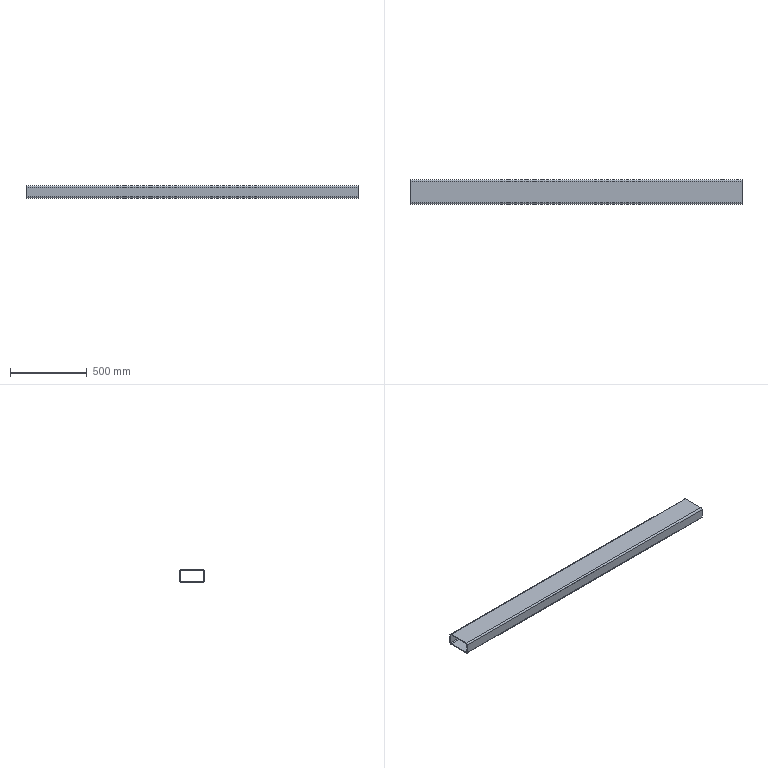Part | SolidWorks | features BaseBody 1 | 1 solid | 26 faces | box 2160 x 160 x 80 mm | volume 4825859 mm3 | cylinder 16 | plane 10 | commonest cylinder face diameters 14 x8 10 x4 20 x4
STEP:
#1=CARTESIAN_POINT('',(1050.,75.,-17.));
#2=VERTEX_POINT('',#1);
#3=CARTESIAN_POINT('',(1050.,75.,-3.));
#4=VERTEX_POINT('',#3);
#5=CARTESIAN_POINT('',(1050.,75.,-10.));
#6=DIRECTION('',(0.,-1.,0.));
#7=DIRECTION('',(0.,0.,-1.));
#8=AXIS2_PLACEMENT_3D('',#5,#6,#7);
#9=CIRCLE('',#8,7.);
#10=EDGE_CURVE('',#2,#4,#9,.T.);
#11=ORIENTED_EDGE('',*,*,#10,.T.);
#12=CARTESIAN_POINT('',(1050.,80.,-3.));
#13=VERTEX_POINT('',#12);
#14=CARTESIAN_POINT('',(1050.,100.,-3.));
#15=DIRECTION('',(0.,1.,0.));
#16=VECTOR('',#15,1000.);
#17=LINE('',#14,#16);
#18=EDGE_CURVE('',#4,#13,#17,.T.);
#19=ORIENTED_EDGE('',*,*,#18,.T.);
#20=CARTESIAN_POINT('',(1050.,80.,-17.));
#21=VERTEX_POINT('',#20);
#22=CARTESIAN_POINT('',(1050.,80.,-10.));
#23=DIRECTION('',(0.,-1.,0.));
#24=DIRECTION('',(0.,0.,-1.));
#25=AXIS2_PLACEMENT_3D('',#22,#23,#24);
#26=CIRCLE('',#25,7.);
#27=EDGE_CURVE('',#21,#13,#26,.T.);
#28=ORIENTED_EDGE('',*,*,#27,.F.);
#29=CARTESIAN_POINT('',(1050.,100.,-17.));
#30=DIRECTION('',(0.,1.,0.));
#31=VECTOR('',#30,1000.);
#32=LINE('',#29,#31);
#33=EDGE_CURVE('',#2,#21,#32,.T.);
#34=ORIENTED_EDGE('',*,*,#33,.F.);
#35=EDGE_LOOP('',(#11,#19,#28,#34));
#36=FACE_OUTER_BOUND('',#35,.T.);
#37=CARTESIAN_POINT('',(1050.,100.,-10.));
#38=DIRECTION('',(0.,1.,0.));
#39=DIRECTION('',(0.,0.,-1.));
#40=AXIS2_PLACEMENT_3D('',#37,#38,#39);
#41=CYLINDRICAL_SURFACE('',#40,7.);
#42=ADVANCED_FACE('',(#36),#41,.F.);
#43=CARTESIAN_POINT('',(950.,75.,-17.));
#44=VERTEX_POINT('',#43);
#45=CARTESIAN_POINT('',(950.,75.,-3.));
#46=VERTEX_POINT('',#45);
#47=CARTESIAN_POINT('',(950.,75.,-10.));
#48=DIRECTION('',(0.,-1.,0.));
#49=DIRECTION('',(0.,0.,-1.));
#50=AXIS2_PLACEMENT_3D('',#47,#48,#49);
#51=CIRCLE('',#50,7.);
#52=EDGE_CURVE('',#44,#46,#51,.T.);
#53=ORIENTED_EDGE('',*,*,#52,.T.);
#54=CARTESIAN_POINT('',(950.,80.,-3.));
#55=VERTEX_POINT('',#54);
#56=CARTESIAN_POINT('',(950.,100.,-3.));
#57=DIRECTION('',(0.,1.,0.));
#58=VECTOR('',#57,1000.);
#59=LINE('',#56,#58);
#60=EDGE_CURVE('',#46,#55,#59,.T.);
#61=ORIENTED_EDGE('',*,*,#60,.T.);
#62=CARTESIAN_POINT('',(950.,80.,-17.));
#63=VERTEX_POINT('',#62);
#64=CARTESIAN_POINT('',(950.,80.,-10.));
#65=DIRECTION('',(0.,-1.,0.));
#66=DIRECTION('',(0.,0.,-1.));
#67=AXIS2_PLACEMENT_3D('',#64,#65,#66);
#68=CIRCLE('',#67,7.);
#69=EDGE_CURVE('',#63,#55,#68,.T.);
#70=ORIENTED_EDGE('',*,*,#69,.F.);
#71=CARTESIAN_POINT('',(950.,100.,-17.));
#72=DIRECTION('',(0.,1.,0.));
#73=VECTOR('',#72,1000.);
#74=LINE('',#71,#73);
#75=EDGE_CURVE('',#44,#63,#74,.T.);
#76=ORIENTED_EDGE('',*,*,#75,.F.);
#77=EDGE_LOOP('',(#53,#61,#70,#76));
#78=FACE_OUTER_BOUND('',#77,.T.);
#79=CARTESIAN_POINT('',(950.,100.,-10.));
#80=DIRECTION('',(0.,1.,0.));
#81=DIRECTION('',(0.,0.,-1.));
#82=AXIS2_PLACEMENT_3D('',#79,#80,#81);
#83=CYLINDRICAL_SURFACE('',#82,7.);
#84=ADVANCED_FACE('',(#78),#83,.F.);
#85=CARTESIAN_POINT('',(-220.,75.,-17.));
#86=VERTEX_POINT('',#85);
#87=CARTESIAN_POINT('',(-220.,75.,-3.));
#88=VERTEX_POINT('',#87);
#89=CARTESIAN_POINT('',(-220.,75.,-10.));
#90=DIRECTION('',(0.,-1.,0.));
#91=DIRECTION('',(0.,0.,-1.));
#92=AXIS2_PLACEMENT_3D('',#89,#90,#91);
#93=CIRCLE('',#92,7.);
#94=EDGE_CURVE('',#86,#88,#93,.T.);
#95=ORIENTED_EDGE('',*,*,#94,.T.);
#96=CARTESIAN_POINT('',(-220.,80.,-3.));
#97=VERTEX_POINT('',#96);
#98=CARTESIAN_POINT('',(-220.,100.,-3.));
#99=DIRECTION('',(0.,1.,0.));
#100=VECTOR('',#99,1000.);
#101=LINE('',#98,#100);
#102=EDGE_CURVE('',#88,#97,#101,.T.);
#103=ORIENTED_EDGE('',*,*,#102,.T.);
#104=CARTESIAN_POINT('',(-220.,80.,-17.));
#105=VERTEX_POINT('',#104);
#106=CARTESIAN_POINT('',(-220.,80.,-10.));
#107=DIRECTION('',(0.,-1.,0.));
#108=DIRECTION('',(0.,0.,-1.));
#109=AXIS2_PLACEMENT_3D('',#106,#107,#108);
#110=CIRCLE('',#109,7.);
#111=EDGE_CURVE('',#105,#97,#110,.T.);
#112=ORIENTED_EDGE('',*,*,#111,.F.);
#113=CARTESIAN_POINT('',(-220.,100.,-17.));
#114=DIRECTION('',(0.,1.,0.));
#115=VECTOR('',#114,1000.);
#116=LINE('',#113,#115);
#117=EDGE_CURVE('',#86,#105,#116,.T.);
#118=ORIENTED_EDGE('',*,*,#117,.F.);
#119=EDGE_LOOP('',(#95,#103,#112,#118));
#120=FACE_OUTER_BOUND('',#119,.T.);
#121=CARTESIAN_POINT('',(-220.,100.,-10.));
#122=DIRECTION('',(0.,1.,0.));
#123=DIRECTION('',(0.,0.,-1.));
#124=AXIS2_PLACEMENT_3D('',#121,#122,#123);
#125=CYLINDRICAL_SURFACE('',#124,7.);
#126=ADVANCED_FACE('',(#120),#125,.F.);
#127=CARTESIAN_POINT('',(-320.,75.,-17.));
#128=VERTEX_POINT('',#127);
#129=CARTESIAN_POINT('',(-320.,75.,-3.));
#130=VERTEX_POINT('',#129);
#131=CARTESIAN_POINT('',(-320.,75.,-10.));
#132=DIRECTION('',(0.,-1.,0.));
#133=DIRECTION('',(0.,0.,-1.));
#134=AXIS2_PLACEMENT_3D('',#131,#132,#133);
#135=CIRCLE('',#134,7.);
#136=EDGE_CURVE('',#128,#130,#135,.T.);
#137=ORIENTED_EDGE('',*,*,#136,.T.);
#138=CARTESIAN_POINT('',(-320.,80.,-3.));
#139=VERTEX_POINT('',#138);
#140=CARTESIAN_POINT('',(-320.,100.,-3.));
#141=DIRECTION('',(0.,1.,0.));
#142=VECTOR('',#141,1000.);
#143=LINE('',#140,#142);
#144=EDGE_CURVE('',#130,#139,#143,.T.);
#145=ORIENTED_EDGE('',*,*,#144,.T.);
#146=CARTESIAN_POINT('',(-320.,80.,-17.));
#147=VERTEX_POINT('',#146);
#148=CARTESIAN_POINT('',(-320.,80.,-10.));
#149=DIRECTION('',(0.,-1.,0.));
#150=DIRECTION('',(0.,0.,-1.));
#151=AXIS2_PLACEMENT_3D('',#148,#149,#150);
#152=CIRCLE('',#151,7.);
#153=EDGE_CURVE('',#147,#139,#152,.T.);
#154=ORIENTED_EDGE('',*,*,#153,.F.);
#155=CARTESIAN_POINT('',(-320.,100.,-17.));
#156=DIRECTION('',(0.,1.,0.));
#157=VECTOR('',#156,1000.);
#158=LINE('',#155,#157);
#159=EDGE_CURVE('',#128,#147,#158,.T.);
#160=ORIENTED_EDGE('',*,*,#159,.F.);
#161=EDGE_LOOP('',(#137,#145,#154,#160));
#162=FACE_OUTER_BOUND('',#161,.T.);
#163=CARTESIAN_POINT('',(-320.,100.,-10.));
#164=DIRECTION('',(0.,1.,0.));
#165=DIRECTION('',(0.,0.,-1.));
#166=AXIS2_PLACEMENT_3D('',#163,#164,#165);
#167=CYLINDRICAL_SURFACE('',#166,7.);
#168=ADVANCED_FACE('',(#162),#167,.F.);
#169=CARTESIAN_POINT('',(-1080.,70.,-40.));
#170=VERTEX_POINT('',#169);
#171=CARTESIAN_POINT('',(-1080.,80.,-30.));
#172=VERTEX_POINT('',#171);
#173=CARTESIAN_POINT('',(-1080.,70.,-30.));
#174=DIRECTION('',(1.,0.,0.));
#175=DIRECTION('',(0.,0.,-1.));
#176=AXIS2_PLACEMENT_3D('',#173,#174,#175);
#177=CIRCLE('',#176,10.);
#178=EDGE_CURVE('',#170,#172,#177,.T.);
#179=ORIENTED_EDGE('',*,*,#178,.T.);
#180=CARTESIAN_POINT('',(1080.,80.,-30.));
#181=VERTEX_POINT('',#180);
#182=CARTESIAN_POINT('',(1080.,80.,-30.));
#183=DIRECTION('',(-1.,0.,0.));
#184=VECTOR('',#183,1000.);
#185=LINE('',#182,#184);
#186=EDGE_CURVE('',#181,#172,#185,.T.);
#187=ORIENTED_EDGE('',*,*,#186,.F.);
#188=CARTESIAN_POINT('',(1080.,70.,-40.));
#189=VERTEX_POINT('',#188);
#190=CARTESIAN_POINT('',(1080.,70.,-30.));
#191=DIRECTION('',(1.,0.,0.));
#192=DIRECTION('',(0.,0.,-1.));
#193=AXIS2_PLACEMENT_3D('',#190,#191,#192);
#194=CIRCLE('',#193,10.);
#195=EDGE_CURVE('',#189,#181,#194,.T.);
#196=ORIENTED_EDGE('',*,*,#195,.F.);
#197=CARTESIAN_POINT('',(1080.,70.,-40.));
#198=DIRECTION('',(-1.,0.,0.));
#199=VECTOR('',#198,1000.);
#200=LINE('',#197,#199);
#201=EDGE_CURVE('',#189,#170,#200,.T.);
#202=ORIENTED_EDGE('',*,*,#201,.T.);
#203=EDGE_LOOP('',(#179,#187,#196,#202));
#204=FACE_OUTER_BOUND('',#203,.T.);
#205=CARTESIAN_POINT('',(1080.,70.,-30.));
#206=DIRECTION('',(-1.,0.,0.));
#207=DIRECTION('',(0.,0.,1.));
#208=AXIS2_PLACEMENT_3D('',#205,#206,#207);
#209=CYLINDRICAL_SURFACE('',#208,10.);
#210=ADVANCED_FACE('',(#204),#209,.T.);
#211=ORIENTED_EDGE('',*,*,#27,.T.);
#212=CARTESIAN_POINT('',(1050.,80.,-10.));
#213=DIRECTION('',(0.,-1.,0.));
#214=DIRECTION('',(0.,0.,-1.));
#215=AXIS2_PLACEMENT_3D('',#212,#213,#214);
#216=CIRCLE('',#215,7.);
#217=EDGE_CURVE('',#13,#21,#216,.T.);
#218=ORIENTED_EDGE('',*,*,#217,.T.);
#219=EDGE_LOOP('',(#211,#218));
#220=FACE_BOUND('',#219,.T.);
#221=ORIENTED_EDGE('',*,*,#69,.T.);
#222=CARTESIAN_POINT('',(950.,80.,-10.));
#223=DIRECTION('',(0.,-1.,0.));
#224=DIRECTION('',(0.,0.,-1.));
#225=AXIS2_PLACEMENT_3D('',#222,#223,#224);
#226=CIRCLE('',#225,7.);
#227=EDGE_CURVE('',#55,#63,#226,.T.);
#228=ORIENTED_EDGE('',*,*,#227,.T.);
#229=EDGE_LOOP('',(#221,#228));
#230=FACE_BOUND('',#229,.T.);
#231=ORIENTED_EDGE('',*,*,#111,.T.);
#232=CARTESIAN_POINT('',(-220.,80.,-10.));
#233=DIRECTION('',(0.,-1.,0.));
#234=DIRECTION('',(0.,0.,-1.));
#235=AXIS2_PLACEMENT_3D('',#232,#233,#234);
#236=CIRCLE('',#235,7.);
#237=EDGE_CURVE('',#97,#105,#236,.T.);
#238=ORIENTED_EDGE('',*,*,#237,.T.);
#239=EDGE_LOOP('',(#231,#238));
#240=FACE_BOUND('',#239,.T.);
#241=ORIENTED_EDGE('',*,*,#153,.T.);
#242=CARTESIAN_POINT('',(-320.,80.,-10.));
#243=DIRECTION('',(0.,-1.,0.));
#244=DIRECTION('',(0.,0.,-1.));
#245=AXIS2_PLACEMENT_3D('',#242,#243,#244);
#246=CIRCLE('',#245,7.);
#247=EDGE_CURVE('',#139,#147,#246,.T.);
#248=ORIENTED_EDGE('',*,*,#247,.T.);
#249=EDGE_LOOP('',(#241,#248));
#250=FACE_BOUND('',#249,.T.);
#251=CARTESIAN_POINT('',(-1080.,80.,30.));
#252=VERTEX_POINT('',#251);
#253=CARTESIAN_POINT('',(-1080.,80.,-30.));
#254=DIRECTION('',(0.,0.,1.));
#255=VECTOR('',#254,1000.);
#256=LINE('',#253,#255);
#257=EDGE_CURVE('',#172,#252,#256,.T.);
#258=ORIENTED_EDGE('',*,*,#257,.T.);
#259=CARTESIAN_POINT('',(1080.,80.,30.));
#260=VERTEX_POINT('',#259);
#261=CARTESIAN_POINT('',(1080.,80.,30.));
#262=DIRECTION('',(-1.,0.,0.));
#263=VECTOR('',#262,1000.);
#264=LINE('',#261,#263);
#265=EDGE_CURVE('',#260,#252,#264,.T.);
#266=ORIENTED_EDGE('',*,*,#265,.F.);
#267=CARTESIAN_POINT('',(1080.,80.,-30.));
#268=DIRECTION('',(0.,0.,1.));
#269=VECTOR('',#268,1000.);
#270=LINE('',#267,#269);
#271=EDGE_CURVE('',#181,#260,#270,.T.);
#272=ORIENTED_EDGE('',*,*,#271,.F.);
#273=ORIENTED_EDGE('',*,*,#186,.T.);
#274=EDGE_LOOP('',(#258,#266,#272,#273));
#275=FACE_OUTER_BOUND('',#274,.T.);
#276=CARTESIAN_POINT('',(1080.,80.,-30.));
#277=DIRECTION('',(0.,-1.,0.));
#278=DIRECTION('',(0.,0.,-1.));
#279=AXIS2_PLACEMENT_3D('',#276,#277,#278);
#280=PLANE('',#279);
#281=ADVANCED_FACE('',(#220,#230,#240,#250,#275),#280,.F.);
#282=CARTESIAN_POINT('',(-1080.,70.,40.));
#283=VERTEX_POINT('',#282);
#284=CARTESIAN_POINT('',(-1080.,70.,30.));
#285=DIRECTION('',(1.,0.,0.));
#286=DIRECTION('',(0.,0.,-1.));
#287=AXIS2_PLACEMENT_3D('',#284,#285,#286);
#288=CIRCLE('',#287,10.);
#289=EDGE_CURVE('',#252,#283,#288,.T.);
#290=ORIENTED_EDGE('',*,*,#289,.T.);
#291=CARTESIAN_POINT('',(1080.,70.,40.));
#292=VERTEX_POINT('',#291);
#293=CARTESIAN_POINT('',(1080.,70.,40.));
#294=DIRECTION('',(-1.,0.,0.));
#295=VECTOR('',#294,1000.);
#296=LINE('',#293,#295);
#297=EDGE_CURVE('',#292,#283,#296,.T.);
#298=ORIENTED_EDGE('',*,*,#297,.F.);
#299=CARTESIAN_POINT('',(1080.,70.,30.));
#300=DIRECTION('',(1.,0.,0.));
#301=DIRECTION('',(0.,0.,-1.));
#302=AXIS2_PLACEMENT_3D('',#299,#300,#301);
#303=CIRCLE('',#302,10.);
#304=EDGE_CURVE('',#260,#292,#303,.T.);
#305=ORIENTED_EDGE('',*,*,#304,.F.);
#306=ORIENTED_EDGE('',*,*,#265,.T.);
#307=EDGE_LOOP('',(#290,#298,#305,#306));
#308=FACE_OUTER_BOUND('',#307,.T.);
#309=CARTESIAN_POINT('',(1080.,70.,30.));
#310=DIRECTION('',(-1.,0.,0.));
#311=DIRECTION('',(0.,0.,1.));
#312=AXIS2_PLACEMENT_3D('',#309,#310,#311);
#313=CYLINDRICAL_SURFACE('',#312,10.);
#314=ADVANCED_FACE('',(#308),#313,.T.);
#315=CARTESIAN_POINT('',(-1080.,-70.,40.));
#316=VERTEX_POINT('',#315);
#317=CARTESIAN_POINT('',(-1080.,-70.,40.));
#318=DIRECTION('',(0.,-1.,0.));
#319=VECTOR('',#318,1000.);
#320=LINE('',#317,#319);
#321=EDGE_CURVE('',#283,#316,#320,.T.);
#322=ORIENTED_EDGE('',*,*,#321,.T.);
#323=CARTESIAN_POINT('',(1080.,-70.,40.));
#324=VERTEX_POINT('',#323);
#325=CARTESIAN_POINT('',(1080.,-70.,40.));
#326=DIRECTION('',(-1.,0.,0.));
#327=VECTOR('',#326,1000.);
#328=LINE('',#325,#327);
#329=EDGE_CURVE('',#324,#316,#328,.T.);
#330=ORIENTED_EDGE('',*,*,#329,.F.);
#331=CARTESIAN_POINT('',(1080.,-70.,40.));
#332=DIRECTION('',(0.,-1.,0.));
#333=VECTOR('',#332,1000.);
#334=LINE('',#331,#333);
#335=EDGE_CURVE('',#292,#324,#334,.T.);
#336=ORIENTED_EDGE('',*,*,#335,.F.);
#337=ORIENTED_EDGE('',*,*,#297,.T.);
#338=EDGE_LOOP('',(#322,#330,#336,#337));
#339=FACE_OUTER_BOUND('',#338,.T.);
#340=CARTESIAN_POINT('',(1080.,-70.,40.));
#341=DIRECTION('',(0.,0.,-1.));
#342=DIRECTION('',(0.,1.,0.));
#343=AXIS2_PLACEMENT_3D('',#340,#341,#342);
#344=PLANE('',#343);
#345=ADVANCED_FACE('',(#339),#344,.F.);
#346=CARTESIAN_POINT('',(-1080.,-80.,30.));
#347=VERTEX_POINT('',#346);
#348=CARTESIAN_POINT('',(-1080.,-70.,30.));
#349=DIRECTION('',(1.,0.,0.));
#350=DIRECTION('',(0.,0.,-1.));
#351=AXIS2_PLACEMENT_3D('',#348,#349,#350);
#352=CIRCLE('',#351,10.);
#353=EDGE_CURVE('',#316,#347,#352,.T.);
#354=ORIENTED_EDGE('',*,*,#353,.T.);
#355=CARTESIAN_POINT('',(1080.,-80.,30.));
#356=VERTEX_POINT('',#355);
#357=CARTESIAN_POINT('',(1080.,-80.,30.));
#358=DIRECTION('',(-1.,0.,0.));
#359=VECTOR('',#358,1000.);
#360=LINE('',#357,#359);
#361=EDGE_CURVE('',#356,#347,#360,.T.);
#362=ORIENTED_EDGE('',*,*,#361,.F.);
#363=CARTESIAN_POINT('',(1080.,-70.,30.));
#364=DIRECTION('',(1.,0.,0.));
#365=DIRECTION('',(0.,0.,-1.));
#366=AXIS2_PLACEMENT_3D('',#363,#364,#365);
#367=CIRCLE('',#366,10.);
#368=EDGE_CURVE('',#324,#356,#367,.T.);
#369=ORIENTED_EDGE('',*,*,#368,.F.);
#370=ORIENTED_EDGE('',*,*,#329,.T.);
#371=EDGE_LOOP('',(#354,#362,#369,#370));
#372=FACE_OUTER_BOUND('',#371,.T.);
#373=CARTESIAN_POINT('',(1080.,-70.,30.));
#374=DIRECTION('',(-1.,0.,0.));
#375=DIRECTION('',(0.,0.,1.));
#376=AXIS2_PLACEMENT_3D('',#373,#374,#375);
#377=CYLINDRICAL_SURFACE('',#376,10.);
#378=ADVANCED_FACE('',(#372),#377,.T.);
#379=CARTESIAN_POINT('',(-1080.,-80.,-30.));
#380=VERTEX_POINT('',#379);
#381=CARTESIAN_POINT('',(-1080.,-80.,30.));
#382=DIRECTION('',(0.,0.,-1.));
#383=VECTOR('',#382,1000.);
#384=LINE('',#381,#383);
#385=EDGE_CURVE('',#347,#380,#384,.T.);
#386=ORIENTED_EDGE('',*,*,#385,.T.);
#387=CARTESIAN_POINT('',(1080.,-80.,-30.));
#388=VERTEX_POINT('',#387);
#389=CARTESIAN_POINT('',(1080.,-80.,-30.));
#390=DIRECTION('',(-1.,0.,0.));
#391=VECTOR('',#390,1000.);
#392=LINE('',#389,#391);
#393=EDGE_CURVE('',#388,#380,#392,.T.);
#394=ORIENTED_EDGE('',*,*,#393,.F.);
#395=CARTESIAN_POINT('',(1080.,-80.,30.));
#396=DIRECTION('',(0.,0.,-1.));
#397=VECTOR('',#396,1000.);
#398=LINE('',#395,#397);
#399=EDGE_CURVE('',#356,#388,#398,.T.);
#400=ORIENTED_EDGE('',*,*,#399,.F.);
#401=ORIENTED_EDGE('',*,*,#361,.T.);
#402=EDGE_LOOP('',(#386,#394,#400,#401));
#403=FACE_OUTER_BOUND('',#402,.T.);
#404=CARTESIAN_POINT('',(1080.,-80.,30.));
#405=DIRECTION('',(0.,1.,0.));
#406=DIRECTION('',(0.,0.,1.));
#407=AXIS2_PLACEMENT_3D('',#404,#405,#406);
#408=PLANE('',#407);
#409=ADVANCED_FACE('',(#403),#408,.F.);
#410=CARTESIAN_POINT('',(-1080.,-70.,-40.));
#411=VERTEX_POINT('',#410);
#412=CARTESIAN_POINT('',(-1080.,-70.,-30.));
#413=DIRECTION('',(1.,0.,0.));
#414=DIRECTION('',(0.,0.,-1.));
#415=AXIS2_PLACEMENT_3D('',#412,#413,#414);
#416=CIRCLE('',#415,10.);
#417=EDGE_CURVE('',#380,#411,#416,.T.);
#418=ORIENTED_EDGE('',*,*,#417,.T.);
#419=CARTESIAN_POINT('',(1080.,-70.,-40.));
#420=VERTEX_POINT('',#419);
#421=CARTESIAN_POINT('',(1080.,-70.,-40.));
#422=DIRECTION('',(-1.,0.,0.));
#423=VECTOR('',#422,1000.);
#424=LINE('',#421,#423);
#425=EDGE_CURVE('',#420,#411,#424,.T.);
#426=ORIENTED_EDGE('',*,*,#425,.F.);
#427=CARTESIAN_POINT('',(1080.,-70.,-30.));
#428=DIRECTION('',(1.,0.,0.));
#429=DIRECTION('',(0.,0.,-1.));
#430=AXIS2_PLACEMENT_3D('',#427,#428,#429);
#431=CIRCLE('',#430,10.);
#432=EDGE_CURVE('',#388,#420,#431,.T.);
#433=ORIENTED_EDGE('',*,*,#432,.F.);
#434=ORIENTED_EDGE('',*,*,#393,.T.);
#435=EDGE_LOOP('',(#418,#426,#433,#434));
#436=FACE_OUTER_BOUND('',#435,.T.);
#437=CARTESIAN_POINT('',(1080.,-70.,-30.));
#438=DIRECTION('',(-1.,0.,0.));
#439=DIRECTION('',(0.,0.,1.));
#440=AXIS2_PLACEMENT_3D('',#437,#438,#439);
#441=CYLINDRICAL_SURFACE('',#440,10.);
#442=ADVANCED_FACE('',(#436),#441,.T.);
#443=CARTESIAN_POINT('',(-1080.,75.,30.));
#444=VERTEX_POINT('',#443);
#445=CARTESIAN_POINT('',(-1080.,70.,35.));
#446=VERTEX_POINT('',#445);
#447=CARTESIAN_POINT('',(-1080.,70.,30.));
#448=DIRECTION('',(1.,0.,0.));
#449=DIRECTION('',(0.,0.,-1.));
#450=AXIS2_PLACEMENT_3D('',#447,#448,#449);
#451=CIRCLE('',#450,5.);
#452=EDGE_CURVE('',#444,#446,#451,.T.);
#453=ORIENTED_EDGE('',*,*,#452,.F.);
#454=CARTESIAN_POINT('',(1080.,75.,30.));
#455=VERTEX_POINT('',#454);
#456=CARTESIAN_POINT('',(1080.,75.,30.));
#457=DIRECTION('',(-1.,0.,0.));
#458=VECTOR('',#457,1000.);
#459=LINE('',#456,#458);
#460=EDGE_CURVE('',#455,#444,#459,.T.);
#461=ORIENTED_EDGE('',*,*,#460,.F.);
#462=CARTESIAN_POINT('',(1080.,70.,35.));
#463=VERTEX_POINT('',#462);
#464=CARTESIAN_POINT('',(1080.,70.,30.));
#465=DIRECTION('',(1.,0.,0.));
#466=DIRECTION('',(0.,0.,-1.));
#467=AXIS2_PLACEMENT_3D('',#464,#465,#466);
#468=CIRCLE('',#467,5.);
#469=EDGE_CURVE('',#455,#463,#468,.T.);
#470=ORIENTED_EDGE('',*,*,#469,.T.);
#471=CARTESIAN_POINT('',(1080.,70.,35.));
#472=DIRECTION('',(-1.,0.,0.));
#473=VECTOR('',#472,1000.);
#474=LINE('',#471,#473);
#475=EDGE_CURVE('',#463,#446,#474,.T.);
#476=ORIENTED_EDGE('',*,*,#475,.T.);
#477=EDGE_LOOP('',(#453,#461,#470,#476));
#478=FACE_OUTER_BOUND('',#477,.T.);
#479=CARTESIAN_POINT('',(1080.,70.,30.));
#480=DIRECTION('',(-1.,0.,0.));
#481=DIRECTION('',(0.,0.,1.));
#482=AXIS2_PLACEMENT_3D('',#479,#480,#481);
#483=CYLINDRICAL_SURFACE('',#482,5.);
#484=ADVANCED_FACE('',(#478),#483,.F.);
#485=ORIENTED_EDGE('',*,*,#10,.F.);
#486=CARTESIAN_POINT('',(1050.,75.,-10.));
#487=DIRECTION('',(0.,-1.,0.));
#488=DIRECTION('',(0.,0.,-1.));
#489=AXIS2_PLACEMENT_3D('',#486,#487,#488);
#490=CIRCLE('',#489,7.);
#491=EDGE_CURVE('',#4,#2,#490,.T.);
#492=ORIENTED_EDGE('',*,*,#491,.F.);
#493=EDGE_LOOP('',(#485,#492));
#494=FACE_BOUND('',#493,.T.);
#495=ORIENTED_EDGE('',*,*,#52,.F.);
#496=CARTESIAN_POINT('',(950.,75.,-10.));
#497=DIRECTION('',(0.,-1.,0.));
#498=DIRECTION('',(0.,0.,-1.));
#499=AXIS2_PLACEMENT_3D('',#496,#497,#498);
#500=CIRCLE('',#499,7.);
#501=EDGE_CURVE('',#46,#44,#500,.T.);
#502=ORIENTED_EDGE('',*,*,#501,.F.);
#503=EDGE_LOOP('',(#495,#502));
#504=FACE_BOUND('',#503,.T.);
#505=ORIENTED_EDGE('',*,*,#94,.F.);
#506=CARTESIAN_POINT('',(-220.,75.,-10.));
#507=DIRECTION('',(0.,-1.,0.));
#508=DIRECTION('',(0.,0.,-1.));
#509=AXIS2_PLACEMENT_3D('',#506,#507,#508);
#510=CIRCLE('',#509,7.);
#511=EDGE_CURVE('',#88,#86,#510,.T.);
#512=ORIENTED_EDGE('',*,*,#511,.F.);
#513=EDGE_LOOP('',(#505,#512));
#514=FACE_BOUND('',#513,.T.);
#515=ORIENTED_EDGE('',*,*,#136,.F.);
#516=CARTESIAN_POINT('',(-320.,75.,-10.));
#517=DIRECTION('',(0.,-1.,0.));
#518=DIRECTION('',(0.,0.,-1.));
#519=AXIS2_PLACEMENT_3D('',#516,#517,#518);
#520=CIRCLE('',#519,7.);
#521=EDGE_CURVE('',#130,#128,#520,.T.);
#522=ORIENTED_EDGE('',*,*,#521,.F.);
#523=EDGE_LOOP('',(#515,#522));
#524=FACE_BOUND('',#523,.T.);
#525=CARTESIAN_POINT('',(-1080.,75.,-30.));
#526=VERTEX_POINT('',#525);
#527=CARTESIAN_POINT('',(-1080.,75.,-30.));
#528=DIRECTION('',(0.,0.,1.));
#529=VECTOR('',#528,1000.);
#530=LINE('',#527,#529);
#531=EDGE_CURVE('',#526,#444,#530,.T.);
#532=ORIENTED_EDGE('',*,*,#531,.F.);
#533=CARTESIAN_POINT('',(1080.,75.,-30.));
#534=VERTEX_POINT('',#533);
#535=CARTESIAN_POINT('',(1080.,75.,-30.));
#536=DIRECTION('',(-1.,0.,0.));
#537=VECTOR('',#536,1000.);
#538=LINE('',#535,#537);
#539=EDGE_CURVE('',#534,#526,#538,.T.);
#540=ORIENTED_EDGE('',*,*,#539,.F.);
#541=CARTESIAN_POINT('',(1080.,75.,-30.));
#542=DIRECTION('',(0.,0.,1.));
#543=VECTOR('',#542,1000.);
#544=LINE('',#541,#543);
#545=EDGE_CURVE('',#534,#455,#544,.T.);
#546=ORIENTED_EDGE('',*,*,#545,.T.);
#547=ORIENTED_EDGE('',*,*,#460,.T.);
#548=EDGE_LOOP('',(#532,#540,#546,#547));
#549=FACE_OUTER_BOUND('',#548,.T.);
#550=CARTESIAN_POINT('',(1080.,75.,-30.));
#551=DIRECTION('',(0.,-1.,0.));
#552=DIRECTION('',(0.,0.,-1.));
#553=AXIS2_PLACEMENT_3D('',#550,#551,#552);
#554=PLANE('',#553);
#555=ADVANCED_FACE('',(#494,#504,#514,#524,#549),#554,.T.);
#556=CARTESIAN_POINT('',(-1080.,70.,-35.));
#557=VERTEX_POINT('',#556);
#558=CARTESIAN_POINT('',(-1080.,70.,-30.));
#559=DIRECTION('',(1.,0.,0.));
#560=DIRECTION('',(0.,0.,-1.));
#561=AXIS2_PLACEMENT_3D('',#558,#559,#560);
#562=CIRCLE('',#561,5.);
#563=EDGE_CURVE('',#557,#526,#562,.T.);
#564=ORIENTED_EDGE('',*,*,#563,.F.);
#565=CARTESIAN_POINT('',(1080.,70.,-35.));
#566=VERTEX_POINT('',#565);
#567=CARTESIAN_POINT('',(1080.,70.,-35.));
#568=DIRECTION('',(-1.,0.,0.));
#569=VECTOR('',#568,1000.);
#570=LINE('',#567,#569);
#571=EDGE_CURVE('',#566,#557,#570,.T.);
#572=ORIENTED_EDGE('',*,*,#571,.F.);
#573=CARTESIAN_POINT('',(1080.,70.,-30.));
#574=DIRECTION('',(1.,0.,0.));
#575=DIRECTION('',(0.,0.,-1.));
#576=AXIS2_PLACEMENT_3D('',#573,#574,#575);
#577=CIRCLE('',#576,5.);
#578=EDGE_CURVE('',#566,#534,#577,.T.);
#579=ORIENTED_EDGE('',*,*,#578,.T.);
#580=ORIENTED_EDGE('',*,*,#539,.T.);
#581=EDGE_LOOP('',(#564,#572,#579,#580));
#582=FACE_OUTER_BOUND('',#581,.T.);
#583=CARTESIAN_POINT('',(1080.,70.,-30.));
#584=DIRECTION('',(-1.,0.,0.));
#585=DIRECTION('',(0.,0.,1.));
#586=AXIS2_PLACEMENT_3D('',#583,#584,#585);
#587=CYLINDRICAL_SURFACE('',#586,5.);
#588=ADVANCED_FACE('',(#582),#587,.F.);
#589=CARTESIAN_POINT('',(-1080.,-70.,-35.));
#590=VERTEX_POINT('',#589);
#591=CARTESIAN_POINT('',(-1080.,70.,-35.));
#592=DIRECTION('',(0.,1.,0.));
#593=VECTOR('',#592,1000.);
#594=LINE('',#591,#593);
#595=EDGE_CURVE('',#590,#557,#594,.T.);
#596=ORIENTED_EDGE('',*,*,#595,.F.);
#597=CARTESIAN_POINT('',(1080.,-70.,-35.));
#598=VERTEX_POINT('',#597);
#599=CARTESIAN_POINT('',(1080.,-70.,-35.));
#600=DIRECTION('',(-1.,0.,0.));
#601=VECTOR('',#600,1000.);
#602=LINE('',#599,#601);
#603=EDGE_CURVE('',#598,#590,#602,.T.);
#604=ORIENTED_EDGE('',*,*,#603,.F.);
#605=CARTESIAN_POINT('',(1080.,70.,-35.));
#606=DIRECTION('',(0.,1.,0.));
#607=VECTOR('',#606,1000.);
#608=LINE('',#605,#607);
#609=EDGE_CURVE('',#598,#566,#608,.T.);
#610=ORIENTED_EDGE('',*,*,#609,.T.);
#611=ORIENTED_EDGE('',*,*,#571,.T.);
#612=EDGE_LOOP('',(#596,#604,#610,#611));
#613=FACE_OUTER_BOUND('',#612,.T.);
#614=CARTESIAN_POINT('',(1080.,70.,-35.));
#615=DIRECTION('',(0.,0.,1.));
#616=DIRECTION('',(1.,0.,0.));
#617=AXIS2_PLACEMENT_3D('',#614,#615,#616);
#618=PLANE('',#617);
#619=ADVANCED_FACE('',(#613),#618,.T.);
#620=CARTESIAN_POINT('',(-1080.,-75.,-30.));
#621=VERTEX_POINT('',#620);
#622=CARTESIAN_POINT('',(-1080.,-70.,-30.));
#623=DIRECTION('',(1.,0.,0.));
#624=DIRECTION('',(0.,0.,-1.));
#625=AXIS2_PLACEMENT_3D('',#622,#623,#624);
#626=CIRCLE('',#625,5.);
#627=EDGE_CURVE('',#621,#590,#626,.T.);
#628=ORIENTED_EDGE('',*,*,#627,.F.);
#629=CARTESIAN_POINT('',(1080.,-75.,-30.));
#630=VERTEX_POINT('',#629);
#631=CARTESIAN_POINT('',(1080.,-75.,-30.));
#632=DIRECTION('',(-1.,0.,0.));
#633=VECTOR('',#632,1000.);
#634=LINE('',#631,#633);
#635=EDGE_CURVE('',#630,#621,#634,.T.);
#636=ORIENTED_EDGE('',*,*,#635,.F.);
#637=CARTESIAN_POINT('',(1080.,-70.,-30.));
#638=DIRECTION('',(1.,0.,0.));
#639=DIRECTION('',(0.,0.,-1.));
#640=AXIS2_PLACEMENT_3D('',#637,#638,#639);
#641=CIRCLE('',#640,5.);
#642=EDGE_CURVE('',#630,#598,#641,.T.);
#643=ORIENTED_EDGE('',*,*,#642,.T.);
#644=ORIENTED_EDGE('',*,*,#603,.T.);
#645=EDGE_LOOP('',(#628,#636,#643,#644));
#646=FACE_OUTER_BOUND('',#645,.T.);
#647=CARTESIAN_POINT('',(1080.,-70.,-30.));
#648=DIRECTION('',(-1.,0.,0.));
#649=DIRECTION('',(0.,0.,1.));
#650=AXIS2_PLACEMENT_3D('',#647,#648,#649);
#651=CYLINDRICAL_SURFACE('',#650,5.);
#652=ADVANCED_FACE('',(#646),#651,.F.);
#653=CARTESIAN_POINT('',(-1080.,-75.,30.));
#654=VERTEX_POINT('',#653);
#655=CARTESIAN_POINT('',(-1080.,-75.,30.));
#656=DIRECTION('',(0.,0.,-1.));
#657=VECTOR('',#656,1000.);
#658=LINE('',#655,#657);
#659=EDGE_CURVE('',#654,#621,#658,.T.);
#660=ORIENTED_EDGE('',*,*,#659,.F.);
#661=CARTESIAN_POINT('',(1080.,-75.,30.));
#662=VERTEX_POINT('',#661);
#663=CARTESIAN_POINT('',(1080.,-75.,30.));
#664=DIRECTION('',(-1.,0.,0.));
#665=VECTOR('',#664,1000.);
#666=LINE('',#663,#665);
#667=EDGE_CURVE('',#662,#654,#666,.T.);
#668=ORIENTED_EDGE('',*,*,#667,.F.);
#669=CARTESIAN_POINT('',(1080.,-75.,30.));
#670=DIRECTION('',(0.,0.,-1.));
#671=VECTOR('',#670,1000.);
#672=LINE('',#669,#671);
#673=EDGE_CURVE('',#662,#630,#672,.T.);
#674=ORIENTED_EDGE('',*,*,#673,.T.);
#675=ORIENTED_EDGE('',*,*,#635,.T.);
#676=EDGE_LOOP('',(#660,#668,#674,#675));
#677=FACE_OUTER_BOUND('',#676,.T.);
#678=CARTESIAN_POINT('',(1080.,-75.,30.));
#679=DIRECTION('',(0.,1.,0.));
#680=DIRECTION('',(0.,0.,1.));
#681=AXIS2_PLACEMENT_3D('',#678,#679,#680);
#682=PLANE('',#681);
#683=ADVANCED_FACE('',(#677),#682,.T.);
#684=CARTESIAN_POINT('',(-1080.,-70.,35.));
#685=VERTEX_POINT('',#684);
#686=CARTESIAN_POINT('',(-1080.,-70.,30.));
#687=DIRECTION('',(1.,0.,0.));
#688=DIRECTION('',(0.,0.,-1.));
#689=AXIS2_PLACEMENT_3D('',#686,#687,#688);
#690=CIRCLE('',#689,5.);
#691=EDGE_CURVE('',#685,#654,#690,.T.);
#692=ORIENTED_EDGE('',*,*,#691,.F.);
#693=CARTESIAN_POINT('',(1080.,-70.,35.));
#694=VERTEX_POINT('',#693);
#695=CARTESIAN_POINT('',(1080.,-70.,35.));
#696=DIRECTION('',(-1.,0.,0.));
#697=VECTOR('',#696,1000.);
#698=LINE('',#695,#697);
#699=EDGE_CURVE('',#694,#685,#698,.T.);
#700=ORIENTED_EDGE('',*,*,#699,.F.);
#701=CARTESIAN_POINT('',(1080.,-70.,30.));
#702=DIRECTION('',(1.,0.,0.));
#703=DIRECTION('',(0.,0.,-1.));
#704=AXIS2_PLACEMENT_3D('',#701,#702,#703);
#705=CIRCLE('',#704,5.);
#706=EDGE_CURVE('',#694,#662,#705,.T.);
#707=ORIENTED_EDGE('',*,*,#706,.T.);
#708=ORIENTED_EDGE('',*,*,#667,.T.);
#709=EDGE_LOOP('',(#692,#700,#707,#708));
#710=FACE_OUTER_BOUND('',#709,.T.);
#711=CARTESIAN_POINT('',(1080.,-70.,30.));
#712=DIRECTION('',(-1.,0.,0.));
#713=DIRECTION('',(0.,0.,1.));
#714=AXIS2_PLACEMENT_3D('',#711,#712,#713);
#715=CYLINDRICAL_SURFACE('',#714,5.);
#716=ADVANCED_FACE('',(#710),#715,.F.);
#717=CARTESIAN_POINT('',(-1080.,-70.,35.));
#718=DIRECTION('',(0.,-1.,0.));
#719=VECTOR('',#718,1000.);
#720=LINE('',#717,#719);
#721=EDGE_CURVE('',#446,#685,#720,.T.);
#722=ORIENTED_EDGE('',*,*,#721,.F.);
#723=ORIENTED_EDGE('',*,*,#475,.F.);
#724=CARTESIAN_POINT('',(1080.,-70.,35.));
#725=DIRECTION('',(0.,-1.,0.));
#726=VECTOR('',#725,1000.);
#727=LINE('',#724,#726);
#728=EDGE_CURVE('',#463,#694,#727,.T.);
#729=ORIENTED_EDGE('',*,*,#728,.T.);
#730=ORIENTED_EDGE('',*,*,#699,.T.);
#731=EDGE_LOOP('',(#722,#723,#729,#730));
#732=FACE_OUTER_BOUND('',#731,.T.);
#733=CARTESIAN_POINT('',(1080.,-70.,35.));
#734=DIRECTION('',(0.,0.,-1.));
#735=DIRECTION('',(0.,1.,0.));
#736=AXIS2_PLACEMENT_3D('',#733,#734,#735);
#737=PLANE('',#736);
#738=ADVANCED_FACE('',(#732),#737,.T.);
#739=CARTESIAN_POINT('',(-1080.,70.,-40.));
#740=DIRECTION('',(0.,1.,0.));
#741=VECTOR('',#740,1000.);
#742=LINE('',#739,#741);
#743=EDGE_CURVE('',#411,#170,#742,.T.);
#744=ORIENTED_EDGE('',*,*,#743,.T.);
#745=ORIENTED_EDGE('',*,*,#201,.F.);
#746=CARTESIAN_POINT('',(1080.,70.,-40.));
#747=DIRECTION('',(0.,1.,0.));
#748=VECTOR('',#747,1000.);
#749=LINE('',#746,#748);
#750=EDGE_CURVE('',#420,#189,#749,.T.);
#751=ORIENTED_EDGE('',*,*,#750,.F.);
#752=ORIENTED_EDGE('',*,*,#425,.T.);
#753=EDGE_LOOP('',(#744,#745,#751,#752));
#754=FACE_OUTER_BOUND('',#753,.T.);
#755=CARTESIAN_POINT('',(1080.,70.,-40.));
#756=DIRECTION('',(0.,0.,1.));
#757=DIRECTION('',(1.,0.,0.));
#758=AXIS2_PLACEMENT_3D('',#755,#756,#757);
#759=PLANE('',#758);
#760=ADVANCED_FACE('',(#754),#759,.F.);
#761=ORIENTED_EDGE('',*,*,#469,.F.);
#762=ORIENTED_EDGE('',*,*,#545,.F.);
#763=ORIENTED_EDGE('',*,*,#578,.F.);
#764=ORIENTED_EDGE('',*,*,#609,.F.);
#765=ORIENTED_EDGE('',*,*,#642,.F.);
#766=ORIENTED_EDGE('',*,*,#673,.F.);
#767=ORIENTED_EDGE('',*,*,#706,.F.);
#768=ORIENTED_EDGE('',*,*,#728,.F.);
#769=EDGE_LOOP('',(#761,#762,#763,#764,#765,#766,#767,#768));
#770=FACE_BOUND('',#769,.T.);
#771=ORIENTED_EDGE('',*,*,#195,.T.);
#772=ORIENTED_EDGE('',*,*,#271,.T.);
#773=ORIENTED_EDGE('',*,*,#304,.T.);
#774=ORIENTED_EDGE('',*,*,#335,.T.);
#775=ORIENTED_EDGE('',*,*,#368,.T.);
#776=ORIENTED_EDGE('',*,*,#399,.T.);
#777=ORIENTED_EDGE('',*,*,#432,.T.);
#778=ORIENTED_EDGE('',*,*,#750,.T.);
#779=EDGE_LOOP('',(#771,#772,#773,#774,#775,#776,#777,#778));
#780=FACE_OUTER_BOUND('',#779,.T.);
#781=CARTESIAN_POINT('',(1080.,70.,-30.));
#782=DIRECTION('',(1.,0.,0.));
#783=DIRECTION('',(0.,0.,-1.));
#784=AXIS2_PLACEMENT_3D('',#781,#782,#783);
#785=PLANE('',#784);
#786=ADVANCED_FACE('',(#770,#780),#785,.T.);
#787=ORIENTED_EDGE('',*,*,#452,.T.);
#788=ORIENTED_EDGE('',*,*,#721,.T.);
#789=ORIENTED_EDGE('',*,*,#691,.T.);
#790=ORIENTED_EDGE('',*,*,#659,.T.);
#791=ORIENTED_EDGE('',*,*,#627,.T.);
#792=ORIENTED_EDGE('',*,*,#595,.T.);
#793=ORIENTED_EDGE('',*,*,#563,.T.);
#794=ORIENTED_EDGE('',*,*,#531,.T.);
#795=EDGE_LOOP('',(#787,#788,#789,#790,#791,#792,#793,#794));
#796=FACE_BOUND('',#795,.T.);
#797=ORIENTED_EDGE('',*,*,#178,.F.);
#798=ORIENTED_EDGE('',*,*,#743,.F.);
#799=ORIENTED_EDGE('',*,*,#417,.F.);
#800=ORIENTED_EDGE('',*,*,#385,.F.);
#801=ORIENTED_EDGE('',*,*,#353,.F.);
#802=ORIENTED_EDGE('',*,*,#321,.F.);
#803=ORIENTED_EDGE('',*,*,#289,.F.);
#804=ORIENTED_EDGE('',*,*,#257,.F.);
#805=EDGE_LOOP('',(#797,#798,#799,#800,#801,#802,#803,#804));
#806=FACE_OUTER_BOUND('',#805,.T.);
#807=CARTESIAN_POINT('',(-1080.,70.,-30.));
#808=DIRECTION('',(1.,0.,0.));
#809=DIRECTION('',(0.,0.,-1.));
#810=AXIS2_PLACEMENT_3D('',#807,#808,#809);
#811=PLANE('',#810);
#812=ADVANCED_FACE('',(#796,#806),#811,.F.);
#813=ORIENTED_EDGE('',*,*,#144,.F.);
#814=ORIENTED_EDGE('',*,*,#521,.T.);
#815=ORIENTED_EDGE('',*,*,#159,.T.);
#816=ORIENTED_EDGE('',*,*,#247,.F.);
#817=EDGE_LOOP('',(#813,#814,#815,#816));
#818=FACE_OUTER_BOUND('',#817,.T.);
#819=CARTESIAN_POINT('',(-320.,100.,-10.));
#820=DIRECTION('',(0.,1.,0.));
#821=DIRECTION('',(0.,0.,-1.));
#822=AXIS2_PLACEMENT_3D('',#819,#820,#821);
#823=CYLINDRICAL_SURFACE('',#822,7.);
#824=ADVANCED_FACE('',(#818),#823,.F.);
#825=ORIENTED_EDGE('',*,*,#102,.F.);
#826=ORIENTED_EDGE('',*,*,#511,.T.);
#827=ORIENTED_EDGE('',*,*,#117,.T.);
#828=ORIENTED_EDGE('',*,*,#237,.F.);
#829=EDGE_LOOP('',(#825,#826,#827,#828));
#830=FACE_OUTER_BOUND('',#829,.T.);
#831=CARTESIAN_POINT('',(-220.,100.,-10.));
#832=DIRECTION('',(0.,1.,0.));
#833=DIRECTION('',(0.,0.,-1.));
#834=AXIS2_PLACEMENT_3D('',#831,#832,#833);
#835=CYLINDRICAL_SURFACE('',#834,7.);
#836=ADVANCED_FACE('',(#830),#835,.F.);
#837=ORIENTED_EDGE('',*,*,#60,.F.);
#838=ORIENTED_EDGE('',*,*,#501,.T.);
#839=ORIENTED_EDGE('',*,*,#75,.T.);
#840=ORIENTED_EDGE('',*,*,#227,.F.);
#841=EDGE_LOOP('',(#837,#838,#839,#840));
#842=FACE_OUTER_BOUND('',#841,.T.);
#843=CARTESIAN_POINT('',(950.,100.,-10.));
#844=DIRECTION('',(0.,1.,0.));
#845=DIRECTION('',(0.,0.,-1.));
#846=AXIS2_PLACEMENT_3D('',#843,#844,#845);
#847=CYLINDRICAL_SURFACE('',#846,7.);
#848=ADVANCED_FACE('',(#842),#847,.F.);
#849=ORIENTED_EDGE('',*,*,#18,.F.);
#850=ORIENTED_EDGE('',*,*,#491,.T.);
#851=ORIENTED_EDGE('',*,*,#33,.T.);
#852=ORIENTED_EDGE('',*,*,#217,.F.);
#853=EDGE_LOOP('',(#849,#850,#851,#852));
#854=FACE_OUTER_BOUND('',#853,.T.);
#855=CARTESIAN_POINT('',(1050.,100.,-10.));
#856=DIRECTION('',(0.,1.,0.));
#857=DIRECTION('',(0.,0.,-1.));
#858=AXIS2_PLACEMENT_3D('',#855,#856,#857);
#859=CYLINDRICAL_SURFACE('',#858,7.);
#860=ADVANCED_FACE('',(#854),#859,.F.);
#861=CLOSED_SHELL('',(#42,#84,#126,#168,#210,#281,#314,#345,#378,#409,#442,#484,#555,#588,#619,#652,#683,#716,#738,#760,#786,#812,#824,#836,#848,#860));
#862=MANIFOLD_SOLID_BREP('',#861);
#863=CARTESIAN_POINT('',(0.,0.,0.));
#864=DIRECTION('',(0.,0.,1.));
#865=DIRECTION('',(1.,0.,0.));
#866=AXIS2_PLACEMENT_3D('',#863,#864,#865);
#867=(LENGTH_UNIT()NAMED_UNIT(*)SI_UNIT(.MILLI.,.METRE.));
#868=UNCERTAINTY_MEASURE_WITH_UNIT(LENGTH_MEASURE(0.00001),#867,'','');
#869=(NAMED_UNIT(*)PLANE_ANGLE_UNIT()SI_UNIT($,.RADIAN.));
#870=(NAMED_UNIT(*)SI_UNIT($,.STERADIAN.)SOLID_ANGLE_UNIT());
#871=(GEOMETRIC_REPRESENTATION_CONTEXT(3)GLOBAL_UNCERTAINTY_ASSIGNED_CONTEXT((#868))GLOBAL_UNIT_ASSIGNED_CONTEXT((#867,#869,#870))REPRESENTATION_CONTEXT('',''));
#872=ADVANCED_BREP_SHAPE_REPRESENTATION('',(#862,#866),#871);